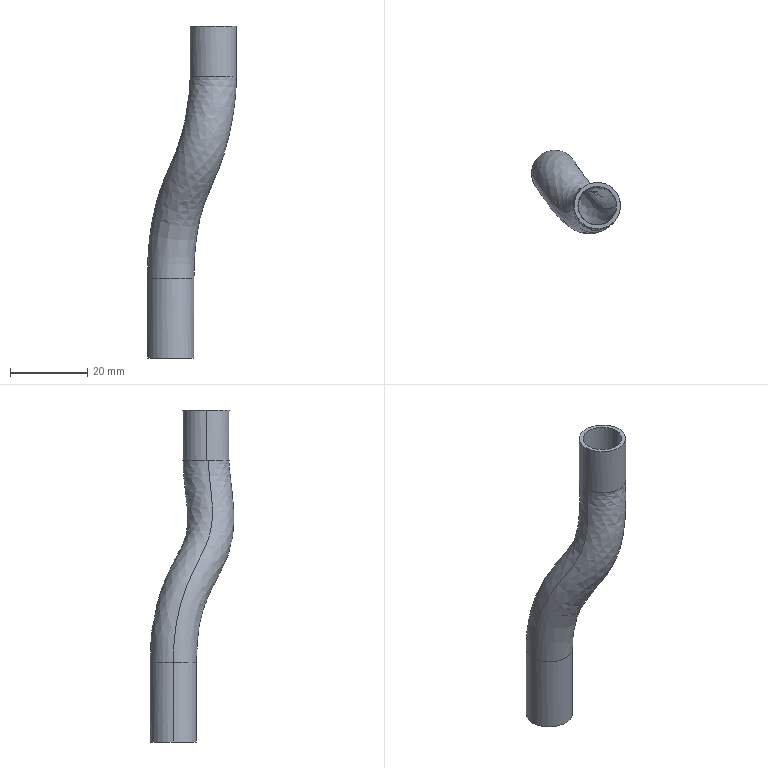Part | SolidWorks | features 3DProfileFeature 2, Sweep 1 | 1 solid | 14 faces | box 23 x 21.644 x 85.817 mm | volume 3078 mm3 | cylinder 8 | spline 4 | plane 2 | commonest cylinder face diameters 10 x4 12 x4